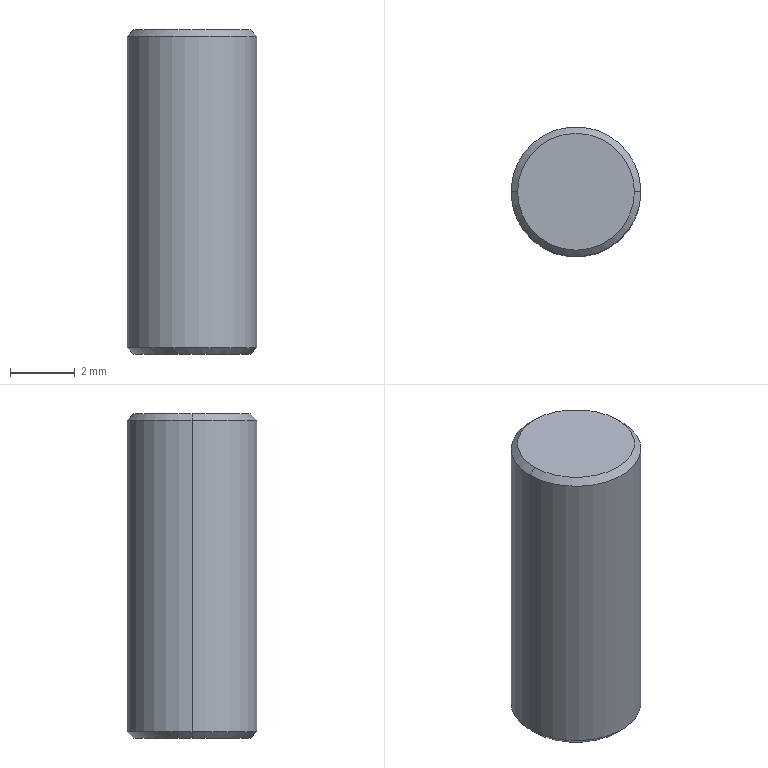Part | STEP file | Needle roller domestic φ4-10-1 | 1 solid | 8 faces | box 4 x 4 x 10 mm | volume 125.178 mm3 | cone 4 | cylinder 2 | plane 2 | commonest cylinder face diameters 4 x2
STEP:
#1=CARTESIAN_POINT('',(-1.8,0.,0.));
#2=VERTEX_POINT('',#1);
#3=CARTESIAN_POINT('',(1.8,0.,0.));
#4=VERTEX_POINT('',#3);
#5=CARTESIAN_POINT('',(0.,0.,0.));
#6=DIRECTION('',(0.,0.,-1.));
#7=DIRECTION('',(1.,0.,0.));
#8=AXIS2_PLACEMENT_3D('',#5,#6,#7);
#9=CIRCLE('',#8,1.8);
#10=EDGE_CURVE('',#2,#4,#9,.T.);
#11=ORIENTED_EDGE('',*,*,#10,.F.);
#12=CARTESIAN_POINT('',(-2.,0.,0.2));
#13=VERTEX_POINT('',#12);
#14=CARTESIAN_POINT('',(-2.,0.,0.2));
#15=DIRECTION('',(-0.7071,0.,0.7071));
#16=VECTOR('',#15,1000.);
#17=LINE('',#14,#16);
#18=EDGE_CURVE('',#2,#13,#17,.T.);
#19=ORIENTED_EDGE('',*,*,#18,.T.);
#20=CARTESIAN_POINT('',(2.,0.,0.2));
#21=VERTEX_POINT('',#20);
#22=CARTESIAN_POINT('',(0.,0.,0.2));
#23=DIRECTION('',(0.,0.,1.));
#24=DIRECTION('',(1.,0.,0.));
#25=AXIS2_PLACEMENT_3D('',#22,#23,#24);
#26=CIRCLE('',#25,2.);
#27=EDGE_CURVE('',#21,#13,#26,.T.);
#28=ORIENTED_EDGE('',*,*,#27,.F.);
#29=CARTESIAN_POINT('',(2.,0.,0.2));
#30=DIRECTION('',(0.7071,0.,0.7071));
#31=VECTOR('',#30,1000.);
#32=LINE('',#29,#31);
#33=EDGE_CURVE('',#4,#21,#32,.T.);
#34=ORIENTED_EDGE('',*,*,#33,.F.);
#35=EDGE_LOOP('',(#11,#19,#28,#34));
#36=FACE_OUTER_BOUND('',#35,.T.);
#37=CARTESIAN_POINT('',(0.,0.,0.2));
#38=DIRECTION('',(0.,0.,1.));
#39=DIRECTION('',(1.,0.,0.));
#40=AXIS2_PLACEMENT_3D('',#37,#38,#39);
#41=CONICAL_SURFACE('',#40,2.,0.7854);
#42=ADVANCED_FACE('',(#36),#41,.T.);
#43=CARTESIAN_POINT('',(1.8,0.,10.));
#44=VERTEX_POINT('',#43);
#45=CARTESIAN_POINT('',(-1.8,0.,10.));
#46=VERTEX_POINT('',#45);
#47=CARTESIAN_POINT('',(0.,0.,10.));
#48=DIRECTION('',(0.,0.,1.));
#49=DIRECTION('',(1.,0.,0.));
#50=AXIS2_PLACEMENT_3D('',#47,#48,#49);
#51=CIRCLE('',#50,1.8);
#52=EDGE_CURVE('',#44,#46,#51,.T.);
#53=ORIENTED_EDGE('',*,*,#52,.F.);
#54=CARTESIAN_POINT('',(2.,0.,9.8));
#55=VERTEX_POINT('',#54);
#56=CARTESIAN_POINT('',(1.8,0.,10.));
#57=DIRECTION('',(0.7071,0.,-0.7071));
#58=VECTOR('',#57,1000.);
#59=LINE('',#56,#58);
#60=EDGE_CURVE('',#44,#55,#59,.T.);
#61=ORIENTED_EDGE('',*,*,#60,.T.);
#62=CARTESIAN_POINT('',(-2.,0.,9.8));
#63=VERTEX_POINT('',#62);
#64=CARTESIAN_POINT('',(0.,0.,9.8));
#65=DIRECTION('',(0.,0.,-1.));
#66=DIRECTION('',(1.,0.,0.));
#67=AXIS2_PLACEMENT_3D('',#64,#65,#66);
#68=CIRCLE('',#67,2.);
#69=EDGE_CURVE('',#63,#55,#68,.T.);
#70=ORIENTED_EDGE('',*,*,#69,.F.);
#71=CARTESIAN_POINT('',(-1.8,0.,10.));
#72=DIRECTION('',(-0.7071,0.,-0.7071));
#73=VECTOR('',#72,1000.);
#74=LINE('',#71,#73);
#75=EDGE_CURVE('',#46,#63,#74,.T.);
#76=ORIENTED_EDGE('',*,*,#75,.F.);
#77=EDGE_LOOP('',(#53,#61,#70,#76));
#78=FACE_OUTER_BOUND('',#77,.T.);
#79=CARTESIAN_POINT('',(0.,0.,10.));
#80=DIRECTION('',(0.,0.,-1.));
#81=DIRECTION('',(-1.,0.,0.));
#82=AXIS2_PLACEMENT_3D('',#79,#80,#81);
#83=CONICAL_SURFACE('',#82,1.8,0.7854);
#84=ADVANCED_FACE('',(#78),#83,.T.);
#85=ORIENTED_EDGE('',*,*,#69,.T.);
#86=CARTESIAN_POINT('',(2.,0.,10.));
#87=DIRECTION('',(0.,0.,-1.));
#88=VECTOR('',#87,1000.);
#89=LINE('',#86,#88);
#90=EDGE_CURVE('',#55,#21,#89,.T.);
#91=ORIENTED_EDGE('',*,*,#90,.T.);
#92=ORIENTED_EDGE('',*,*,#27,.T.);
#93=CARTESIAN_POINT('',(-2.,0.,10.));
#94=DIRECTION('',(0.,0.,-1.));
#95=VECTOR('',#94,1000.);
#96=LINE('',#93,#95);
#97=EDGE_CURVE('',#63,#13,#96,.T.);
#98=ORIENTED_EDGE('',*,*,#97,.F.);
#99=EDGE_LOOP('',(#85,#91,#92,#98));
#100=FACE_OUTER_BOUND('',#99,.T.);
#101=CARTESIAN_POINT('',(0.,0.,10.));
#102=DIRECTION('',(0.,0.,-1.));
#103=DIRECTION('',(-1.,0.,0.));
#104=AXIS2_PLACEMENT_3D('',#101,#102,#103);
#105=CYLINDRICAL_SURFACE('',#104,2.);
#106=ADVANCED_FACE('',(#100),#105,.T.);
#107=ORIENTED_EDGE('',*,*,#90,.F.);
#108=CARTESIAN_POINT('',(0.,0.,9.8));
#109=DIRECTION('',(0.,0.,-1.));
#110=DIRECTION('',(1.,0.,0.));
#111=AXIS2_PLACEMENT_3D('',#108,#109,#110);
#112=CIRCLE('',#111,2.);
#113=EDGE_CURVE('',#55,#63,#112,.T.);
#114=ORIENTED_EDGE('',*,*,#113,.T.);
#115=ORIENTED_EDGE('',*,*,#97,.T.);
#116=CARTESIAN_POINT('',(0.,0.,0.2));
#117=DIRECTION('',(0.,0.,1.));
#118=DIRECTION('',(1.,0.,0.));
#119=AXIS2_PLACEMENT_3D('',#116,#117,#118);
#120=CIRCLE('',#119,2.);
#121=EDGE_CURVE('',#13,#21,#120,.T.);
#122=ORIENTED_EDGE('',*,*,#121,.T.);
#123=EDGE_LOOP('',(#107,#114,#115,#122));
#124=FACE_OUTER_BOUND('',#123,.T.);
#125=CARTESIAN_POINT('',(0.,0.,10.));
#126=DIRECTION('',(0.,0.,-1.));
#127=DIRECTION('',(-1.,0.,0.));
#128=AXIS2_PLACEMENT_3D('',#125,#126,#127);
#129=CYLINDRICAL_SURFACE('',#128,2.);
#130=ADVANCED_FACE('',(#124),#129,.T.);
#131=CARTESIAN_POINT('',(0.,0.,10.));
#132=DIRECTION('',(0.,0.,1.));
#133=DIRECTION('',(1.,0.,0.));
#134=AXIS2_PLACEMENT_3D('',#131,#132,#133);
#135=CIRCLE('',#134,1.8);
#136=EDGE_CURVE('',#46,#44,#135,.T.);
#137=ORIENTED_EDGE('',*,*,#136,.T.);
#138=ORIENTED_EDGE('',*,*,#52,.T.);
#139=EDGE_LOOP('',(#137,#138));
#140=FACE_OUTER_BOUND('',#139,.T.);
#141=CARTESIAN_POINT('',(0.,0.,10.));
#142=DIRECTION('',(0.,0.,1.));
#143=DIRECTION('',(1.,0.,0.));
#144=AXIS2_PLACEMENT_3D('',#141,#142,#143);
#145=PLANE('',#144);
#146=ADVANCED_FACE('',(#140),#145,.T.);
#147=CARTESIAN_POINT('',(0.,0.,0.));
#148=DIRECTION('',(0.,0.,-1.));
#149=DIRECTION('',(1.,0.,0.));
#150=AXIS2_PLACEMENT_3D('',#147,#148,#149);
#151=CIRCLE('',#150,1.8);
#152=EDGE_CURVE('',#4,#2,#151,.T.);
#153=ORIENTED_EDGE('',*,*,#152,.T.);
#154=ORIENTED_EDGE('',*,*,#10,.T.);
#155=EDGE_LOOP('',(#153,#154));
#156=FACE_OUTER_BOUND('',#155,.T.);
#157=CARTESIAN_POINT('',(0.,0.,0.));
#158=DIRECTION('',(0.,0.,1.));
#159=DIRECTION('',(1.,0.,0.));
#160=AXIS2_PLACEMENT_3D('',#157,#158,#159);
#161=PLANE('',#160);
#162=ADVANCED_FACE('',(#156),#161,.F.);
#163=ORIENTED_EDGE('',*,*,#60,.F.);
#164=ORIENTED_EDGE('',*,*,#136,.F.);
#165=ORIENTED_EDGE('',*,*,#75,.T.);
#166=ORIENTED_EDGE('',*,*,#113,.F.);
#167=EDGE_LOOP('',(#163,#164,#165,#166));
#168=FACE_OUTER_BOUND('',#167,.T.);
#169=CARTESIAN_POINT('',(0.,0.,10.));
#170=DIRECTION('',(0.,0.,-1.));
#171=DIRECTION('',(-1.,0.,0.));
#172=AXIS2_PLACEMENT_3D('',#169,#170,#171);
#173=CONICAL_SURFACE('',#172,1.8,0.7854);
#174=ADVANCED_FACE('',(#168),#173,.T.);
#175=ORIENTED_EDGE('',*,*,#18,.F.);
#176=ORIENTED_EDGE('',*,*,#152,.F.);
#177=ORIENTED_EDGE('',*,*,#33,.T.);
#178=ORIENTED_EDGE('',*,*,#121,.F.);
#179=EDGE_LOOP('',(#175,#176,#177,#178));
#180=FACE_OUTER_BOUND('',#179,.T.);
#181=CARTESIAN_POINT('',(0.,0.,0.2));
#182=DIRECTION('',(0.,0.,1.));
#183=DIRECTION('',(1.,0.,0.));
#184=AXIS2_PLACEMENT_3D('',#181,#182,#183);
#185=CONICAL_SURFACE('',#184,2.,0.7854);
#186=ADVANCED_FACE('',(#180),#185,.T.);
#187=CLOSED_SHELL('',(#42,#84,#106,#130,#146,#162,#174,#186));
#188=MANIFOLD_SOLID_BREP('',#187);
#189=CARTESIAN_POINT('',(0.,0.,0.));
#190=DIRECTION('',(0.,0.,1.));
#191=DIRECTION('',(1.,0.,0.));
#192=AXIS2_PLACEMENT_3D('',#189,#190,#191);
#193=(LENGTH_UNIT()NAMED_UNIT(*)SI_UNIT(.MILLI.,.METRE.));
#194=UNCERTAINTY_MEASURE_WITH_UNIT(LENGTH_MEASURE(0.00001),#193,'','');
#195=(NAMED_UNIT(*)PLANE_ANGLE_UNIT()SI_UNIT($,.RADIAN.));
#196=(NAMED_UNIT(*)SI_UNIT($,.STERADIAN.)SOLID_ANGLE_UNIT());
#197=(GEOMETRIC_REPRESENTATION_CONTEXT(3)GLOBAL_UNCERTAINTY_ASSIGNED_CONTEXT((#194))GLOBAL_UNIT_ASSIGNED_CONTEXT((#193,#195,#196))REPRESENTATION_CONTEXT('',''));
#198=ADVANCED_BREP_SHAPE_REPRESENTATION('',(#188,#192),#197);